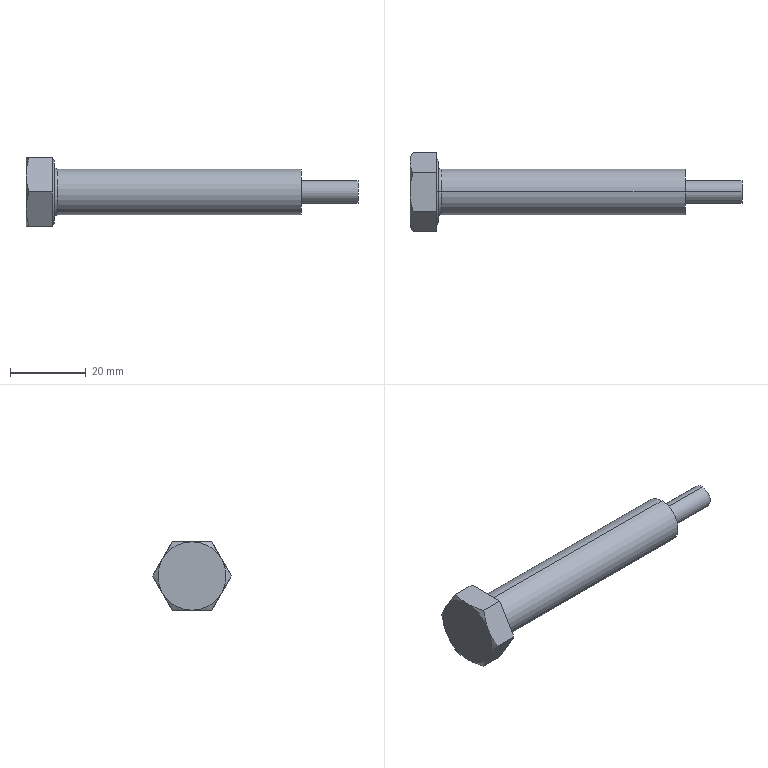Part | SolidWorks | features Chamfer 2, ICE 2, RevCut 2, Revolution 2, Extrusion 1 | 1 solid | 25 faces | box 87.5 x 20.785 x 18 mm | volume 9848 mm3 | plane 11 | cone 8 | cylinder 4 | torus 2 | commonest cylinder face diameters 6 x2 12 x2
STEP:
#1=CARTESIAN_POINT('',(72.5,0.,-3.));
#2=VERTEX_POINT('',#1);
#3=CARTESIAN_POINT('',(72.5,0.,3.));
#4=VERTEX_POINT('',#3);
#5=CARTESIAN_POINT('',(72.5,0.,0.));
#6=DIRECTION('',(1.,0.,0.));
#7=DIRECTION('',(0.,0.,-1.));
#8=AXIS2_PLACEMENT_3D('',#5,#6,#7);
#9=CIRCLE('',#8,3.);
#10=EDGE_CURVE('',#2,#4,#9,.T.);
#11=ORIENTED_EDGE('',*,*,#10,.T.);
#12=CARTESIAN_POINT('',(87.5,0.,3.));
#13=VERTEX_POINT('',#12);
#14=CARTESIAN_POINT('',(72.5,0.,3.));
#15=DIRECTION('',(1.,0.,0.));
#16=VECTOR('',#15,1000.);
#17=LINE('',#14,#16);
#18=EDGE_CURVE('',#4,#13,#17,.T.);
#19=ORIENTED_EDGE('',*,*,#18,.T.);
#20=CARTESIAN_POINT('',(87.5,0.,-3.));
#21=VERTEX_POINT('',#20);
#22=CARTESIAN_POINT('',(87.5,0.,0.));
#23=DIRECTION('',(1.,0.,0.));
#24=DIRECTION('',(0.,0.,-1.));
#25=AXIS2_PLACEMENT_3D('',#22,#23,#24);
#26=CIRCLE('',#25,3.);
#27=EDGE_CURVE('',#21,#13,#26,.T.);
#28=ORIENTED_EDGE('',*,*,#27,.F.);
#29=CARTESIAN_POINT('',(72.5,0.,-3.));
#30=DIRECTION('',(1.,0.,0.));
#31=VECTOR('',#30,1000.);
#32=LINE('',#29,#31);
#33=EDGE_CURVE('',#2,#21,#32,.T.);
#34=ORIENTED_EDGE('',*,*,#33,.F.);
#35=EDGE_LOOP('',(#11,#19,#28,#34));
#36=FACE_OUTER_BOUND('',#35,.T.);
#37=CARTESIAN_POINT('',(72.5,0.,0.));
#38=DIRECTION('',(1.,0.,0.));
#39=DIRECTION('',(0.,0.,-1.));
#40=AXIS2_PLACEMENT_3D('',#37,#38,#39);
#41=CYLINDRICAL_SURFACE('',#40,3.);
#42=ADVANCED_FACE('',(#36),#41,.T.);
#43=CARTESIAN_POINT('',(7.5,0.,8.215));
#44=VERTEX_POINT('',#43);
#45=CARTESIAN_POINT('',(7.5,0.,-8.215));
#46=VERTEX_POINT('',#45);
#47=CARTESIAN_POINT('',(7.5,0.,0.));
#48=DIRECTION('',(-1.,0.,0.));
#49=DIRECTION('',(0.,0.,1.));
#50=AXIS2_PLACEMENT_3D('',#47,#48,#49);
#51=CIRCLE('',#50,8.215);
#52=EDGE_CURVE('',#44,#46,#51,.T.);
#53=ORIENTED_EDGE('',*,*,#52,.T.);
#54=CARTESIAN_POINT('',(6.9,0.,-8.815));
#55=VERTEX_POINT('',#54);
#56=CARTESIAN_POINT('',(6.9,0.,-8.815));
#57=DIRECTION('',(-0.7071,0.,-0.7071));
#58=VECTOR('',#57,1000.);
#59=LINE('',#56,#58);
#60=EDGE_CURVE('',#46,#55,#59,.T.);
#61=ORIENTED_EDGE('',*,*,#60,.T.);
#62=CARTESIAN_POINT('',(6.9,0.,8.815));
#63=VERTEX_POINT('',#62);
#64=CARTESIAN_POINT('',(6.9,0.,0.));
#65=DIRECTION('',(-1.,0.,0.));
#66=DIRECTION('',(0.,0.,1.));
#67=AXIS2_PLACEMENT_3D('',#64,#65,#66);
#68=CIRCLE('',#67,8.815);
#69=EDGE_CURVE('',#63,#55,#68,.T.);
#70=ORIENTED_EDGE('',*,*,#69,.F.);
#71=CARTESIAN_POINT('',(6.9,0.,8.815));
#72=DIRECTION('',(-0.7071,0.,0.7071));
#73=VECTOR('',#72,1000.);
#74=LINE('',#71,#73);
#75=EDGE_CURVE('',#44,#63,#74,.T.);
#76=ORIENTED_EDGE('',*,*,#75,.F.);
#77=EDGE_LOOP('',(#53,#61,#70,#76));
#78=FACE_OUTER_BOUND('',#77,.T.);
#79=CARTESIAN_POINT('',(6.9,0.,0.));
#80=DIRECTION('',(-1.,0.,0.));
#81=DIRECTION('',(0.,0.,1.));
#82=AXIS2_PLACEMENT_3D('',#79,#80,#81);
#83=CONICAL_SURFACE('',#82,8.815,0.7854);
#84=ADVANCED_FACE('',(#78),#83,.T.);
#85=CARTESIAN_POINT('',(7.5,0.,-6.85));
#86=VERTEX_POINT('',#85);
#87=CARTESIAN_POINT('',(7.5,0.,6.85));
#88=VERTEX_POINT('',#87);
#89=CARTESIAN_POINT('',(7.5,0.,0.));
#90=DIRECTION('',(-1.,0.,0.));
#91=DIRECTION('',(0.,0.,1.));
#92=AXIS2_PLACEMENT_3D('',#89,#90,#91);
#93=CIRCLE('',#92,6.85);
#94=EDGE_CURVE('',#86,#88,#93,.T.);
#95=ORIENTED_EDGE('',*,*,#94,.F.);
#96=CARTESIAN_POINT('',(8.35,0.,-6.));
#97=VERTEX_POINT('',#96);
#98=CARTESIAN_POINT('',(8.35,0.,-6.85));
#99=DIRECTION('',(0.,1.,0.));
#100=DIRECTION('',(0.,0.,1.));
#101=AXIS2_PLACEMENT_3D('',#98,#99,#100);
#102=CIRCLE('',#101,0.85);
#103=EDGE_CURVE('',#86,#97,#102,.T.);
#104=ORIENTED_EDGE('',*,*,#103,.T.);
#105=CARTESIAN_POINT('',(8.35,0.,6.));
#106=VERTEX_POINT('',#105);
#107=CARTESIAN_POINT('',(8.35,0.,0.));
#108=DIRECTION('',(-1.,0.,0.));
#109=DIRECTION('',(0.,0.,1.));
#110=AXIS2_PLACEMENT_3D('',#107,#108,#109);
#111=CIRCLE('',#110,6.);
#112=EDGE_CURVE('',#97,#106,#111,.T.);
#113=ORIENTED_EDGE('',*,*,#112,.T.);
#114=CARTESIAN_POINT('',(8.35,0.,6.85));
#115=DIRECTION('',(0.,-1.,0.));
#116=DIRECTION('',(0.,0.,-1.));
#117=AXIS2_PLACEMENT_3D('',#114,#115,#116);
#118=CIRCLE('',#117,0.85);
#119=EDGE_CURVE('',#88,#106,#118,.T.);
#120=ORIENTED_EDGE('',*,*,#119,.F.);
#121=EDGE_LOOP('',(#95,#104,#113,#120));
#122=FACE_OUTER_BOUND('',#121,.T.);
#123=CARTESIAN_POINT('',(8.35,0.,0.));
#124=DIRECTION('',(-1.,0.,0.));
#125=DIRECTION('',(0.,0.,1.));
#126=AXIS2_PLACEMENT_3D('',#123,#124,#125);
#127=TOROIDAL_SURFACE('',#126,6.85,0.85);
#128=ADVANCED_FACE('',(#122),#127,.F.);
#129=CARTESIAN_POINT('',(72.5,0.,-6.));
#130=VERTEX_POINT('',#129);
#131=CARTESIAN_POINT('',(72.5,0.,6.));
#132=VERTEX_POINT('',#131);
#133=CARTESIAN_POINT('',(72.5,0.,0.));
#134=DIRECTION('',(1.,0.,0.));
#135=DIRECTION('',(0.,0.,-1.));
#136=AXIS2_PLACEMENT_3D('',#133,#134,#135);
#137=CIRCLE('',#136,6.);
#138=EDGE_CURVE('',#130,#132,#137,.T.);
#139=ORIENTED_EDGE('',*,*,#138,.F.);
#140=CARTESIAN_POINT('',(7.5,0.,-6.));
#141=DIRECTION('',(-1.,0.,0.));
#142=VECTOR('',#141,1000.);
#143=LINE('',#140,#142);
#144=EDGE_CURVE('',#130,#97,#143,.T.);
#145=ORIENTED_EDGE('',*,*,#144,.T.);
#146=CARTESIAN_POINT('',(8.35,0.,0.));
#147=DIRECTION('',(-1.,0.,0.));
#148=DIRECTION('',(0.,0.,1.));
#149=AXIS2_PLACEMENT_3D('',#146,#147,#148);
#150=CIRCLE('',#149,6.);
#151=EDGE_CURVE('',#106,#97,#150,.T.);
#152=ORIENTED_EDGE('',*,*,#151,.F.);
#153=CARTESIAN_POINT('',(7.5,0.,6.));
#154=DIRECTION('',(-1.,0.,0.));
#155=VECTOR('',#154,1000.);
#156=LINE('',#153,#155);
#157=EDGE_CURVE('',#132,#106,#156,.T.);
#158=ORIENTED_EDGE('',*,*,#157,.F.);
#159=EDGE_LOOP('',(#139,#145,#152,#158));
#160=FACE_OUTER_BOUND('',#159,.T.);
#161=CARTESIAN_POINT('',(7.5,0.,0.));
#162=DIRECTION('',(-1.,0.,0.));
#163=DIRECTION('',(0.,0.,1.));
#164=AXIS2_PLACEMENT_3D('',#161,#162,#163);
#165=CYLINDRICAL_SURFACE('',#164,6.);
#166=ADVANCED_FACE('',(#160),#165,.T.);
#167=ORIENTED_EDGE('',*,*,#144,.F.);
#168=CARTESIAN_POINT('',(72.5,0.,0.));
#169=DIRECTION('',(1.,0.,0.));
#170=DIRECTION('',(0.,0.,-1.));
#171=AXIS2_PLACEMENT_3D('',#168,#169,#170);
#172=CIRCLE('',#171,6.);
#173=EDGE_CURVE('',#132,#130,#172,.T.);
#174=ORIENTED_EDGE('',*,*,#173,.F.);
#175=ORIENTED_EDGE('',*,*,#157,.T.);
#176=ORIENTED_EDGE('',*,*,#112,.F.);
#177=EDGE_LOOP('',(#167,#174,#175,#176));
#178=FACE_OUTER_BOUND('',#177,.T.);
#179=CARTESIAN_POINT('',(7.5,0.,0.));
#180=DIRECTION('',(-1.,0.,0.));
#181=DIRECTION('',(0.,0.,1.));
#182=AXIS2_PLACEMENT_3D('',#179,#180,#181);
#183=CYLINDRICAL_SURFACE('',#182,6.);
#184=ADVANCED_FACE('',(#178),#183,.T.);
#185=CARTESIAN_POINT('',(7.5,0.,0.));
#186=DIRECTION('',(-1.,0.,0.));
#187=DIRECTION('',(0.,0.,1.));
#188=AXIS2_PLACEMENT_3D('',#185,#186,#187);
#189=CIRCLE('',#188,6.85);
#190=EDGE_CURVE('',#88,#86,#189,.T.);
#191=ORIENTED_EDGE('',*,*,#190,.T.);
#192=ORIENTED_EDGE('',*,*,#94,.T.);
#193=EDGE_LOOP('',(#191,#192));
#194=FACE_BOUND('',#193,.T.);
#195=ORIENTED_EDGE('',*,*,#52,.F.);
#196=CARTESIAN_POINT('',(7.5,0.,0.));
#197=DIRECTION('',(-1.,0.,0.));
#198=DIRECTION('',(0.,0.,1.));
#199=AXIS2_PLACEMENT_3D('',#196,#197,#198);
#200=CIRCLE('',#199,8.215);
#201=EDGE_CURVE('',#46,#44,#200,.T.);
#202=ORIENTED_EDGE('',*,*,#201,.F.);
#203=EDGE_LOOP('',(#195,#202));
#204=FACE_OUTER_BOUND('',#203,.T.);
#205=CARTESIAN_POINT('',(7.5,5.196,-9.));
#206=DIRECTION('',(1.,0.,0.));
#207=DIRECTION('',(0.,0.,-1.));
#208=AXIS2_PLACEMENT_3D('',#205,#206,#207);
#209=PLANE('',#208);
#210=ADVANCED_FACE('',(#194,#204),#209,.T.);
#211=ORIENTED_EDGE('',*,*,#103,.F.);
#212=ORIENTED_EDGE('',*,*,#190,.F.);
#213=ORIENTED_EDGE('',*,*,#119,.T.);
#214=ORIENTED_EDGE('',*,*,#151,.T.);
#215=EDGE_LOOP('',(#211,#212,#213,#214));
#216=FACE_OUTER_BOUND('',#215,.T.);
#217=CARTESIAN_POINT('',(8.35,0.,0.));
#218=DIRECTION('',(-1.,0.,0.));
#219=DIRECTION('',(0.,0.,1.));
#220=AXIS2_PLACEMENT_3D('',#217,#218,#219);
#221=TOROIDAL_SURFACE('',#220,6.85,0.85);
#222=ADVANCED_FACE('',(#216),#221,.F.);
#223=ORIENTED_EDGE('',*,*,#69,.T.);
#224=CARTESIAN_POINT('',(6.9,0.,0.));
#225=DIRECTION('',(-1.,0.,0.));
#226=DIRECTION('',(0.,0.,1.));
#227=AXIS2_PLACEMENT_3D('',#224,#225,#226);
#228=CIRCLE('',#227,8.815);
#229=EDGE_CURVE('',#55,#63,#228,.T.);
#230=ORIENTED_EDGE('',*,*,#229,.T.);
#231=EDGE_LOOP('',(#223,#230));
#232=FACE_BOUND('',#231,.T.);
#233=CARTESIAN_POINT('',(6.9,-5.196,-9.));
#234=VERTEX_POINT('',#233);
#235=CARTESIAN_POINT('',(6.9,5.196,-9.));
#236=VERTEX_POINT('',#235);
#237=CARTESIAN_POINT('',(6.9,-5.196,-9.));
#238=DIRECTION('',(0.,1.,0.));
#239=VECTOR('',#238,1000.);
#240=LINE('',#237,#239);
#241=EDGE_CURVE('',#234,#236,#240,.T.);
#242=ORIENTED_EDGE('',*,*,#241,.T.);
#243=CARTESIAN_POINT('',(6.9,10.392,0.));
#244=VERTEX_POINT('',#243);
#245=CARTESIAN_POINT('',(6.9,5.196,-9.));
#246=DIRECTION('',(0.,0.5,0.866));
#247=VECTOR('',#246,1000.);
#248=LINE('',#245,#247);
#249=EDGE_CURVE('',#236,#244,#248,.T.);
#250=ORIENTED_EDGE('',*,*,#249,.T.);
#251=CARTESIAN_POINT('',(6.9,5.196,9.));
#252=VERTEX_POINT('',#251);
#253=CARTESIAN_POINT('',(6.9,10.392,0.));
#254=DIRECTION('',(0.,-0.5,0.866));
#255=VECTOR('',#254,1000.);
#256=LINE('',#253,#255);
#257=EDGE_CURVE('',#244,#252,#256,.T.);
#258=ORIENTED_EDGE('',*,*,#257,.T.);
#259=CARTESIAN_POINT('',(6.9,-5.196,9.));
#260=VERTEX_POINT('',#259);
#261=CARTESIAN_POINT('',(6.9,5.196,9.));
#262=DIRECTION('',(0.,-1.,0.));
#263=VECTOR('',#262,1000.);
#264=LINE('',#261,#263);
#265=EDGE_CURVE('',#252,#260,#264,.T.);
#266=ORIENTED_EDGE('',*,*,#265,.T.);
#267=CARTESIAN_POINT('',(6.9,-10.392,0.));
#268=VERTEX_POINT('',#267);
#269=CARTESIAN_POINT('',(6.9,-5.196,9.));
#270=DIRECTION('',(0.,-0.5,-0.866));
#271=VECTOR('',#270,1000.);
#272=LINE('',#269,#271);
#273=EDGE_CURVE('',#260,#268,#272,.T.);
#274=ORIENTED_EDGE('',*,*,#273,.T.);
#275=CARTESIAN_POINT('',(6.9,-10.392,0.));
#276=DIRECTION('',(0.,0.5,-0.866));
#277=VECTOR('',#276,1000.);
#278=LINE('',#275,#277);
#279=EDGE_CURVE('',#268,#234,#278,.T.);
#280=ORIENTED_EDGE('',*,*,#279,.T.);
#281=EDGE_LOOP('',(#242,#250,#258,#266,#274,#280));
#282=FACE_OUTER_BOUND('',#281,.T.);
#283=CARTESIAN_POINT('',(6.9,-8.815,0.));
#284=DIRECTION('',(1.,0.,0.));
#285=DIRECTION('',(0.,0.,-1.));
#286=AXIS2_PLACEMENT_3D('',#283,#284,#285);
#287=PLANE('',#286);
#288=ADVANCED_FACE('',(#232,#282),#287,.T.);
#289=ORIENTED_EDGE('',*,*,#60,.F.);
#290=ORIENTED_EDGE('',*,*,#201,.T.);
#291=ORIENTED_EDGE('',*,*,#75,.T.);
#292=ORIENTED_EDGE('',*,*,#229,.F.);
#293=EDGE_LOOP('',(#289,#290,#291,#292));
#294=FACE_OUTER_BOUND('',#293,.T.);
#295=CARTESIAN_POINT('',(6.9,0.,0.));
#296=DIRECTION('',(-1.,0.,0.));
#297=DIRECTION('',(0.,0.,1.));
#298=AXIS2_PLACEMENT_3D('',#295,#296,#297);
#299=CONICAL_SURFACE('',#298,8.815,0.7854);
#300=ADVANCED_FACE('',(#294),#299,.T.);
#301=CARTESIAN_POINT('',(0.,0.,-9.));
#302=VERTEX_POINT('',#301);
#303=CARTESIAN_POINT('',(0.,7.794,-4.5));
#304=VERTEX_POINT('',#303);
#305=CARTESIAN_POINT('',(0.,0.,0.));
#306=DIRECTION('',(1.,0.,0.));
#307=DIRECTION('',(0.,0.,-1.));
#308=AXIS2_PLACEMENT_3D('',#305,#306,#307);
#309=CIRCLE('',#308,9.);
#310=EDGE_CURVE('',#302,#304,#309,.T.);
#311=ORIENTED_EDGE('',*,*,#310,.F.);
#312=CARTESIAN_POINT('',(0.,-7.794,-4.5));
#313=VERTEX_POINT('',#312);
#314=CARTESIAN_POINT('',(0.,0.,0.));
#315=DIRECTION('',(1.,0.,0.));
#316=DIRECTION('',(0.,0.,-1.));
#317=AXIS2_PLACEMENT_3D('',#314,#315,#316);
#318=CIRCLE('',#317,9.);
#319=EDGE_CURVE('',#313,#302,#318,.T.);
#320=ORIENTED_EDGE('',*,*,#319,.F.);
#321=CARTESIAN_POINT('',(0.,-7.794,4.5));
#322=VERTEX_POINT('',#321);
#323=CARTESIAN_POINT('',(0.,0.,0.));
#324=DIRECTION('',(1.,0.,0.));
#325=DIRECTION('',(0.,0.,-1.));
#326=AXIS2_PLACEMENT_3D('',#323,#324,#325);
#327=CIRCLE('',#326,9.);
#328=EDGE_CURVE('',#322,#313,#327,.T.);
#329=ORIENTED_EDGE('',*,*,#328,.F.);
#330=CARTESIAN_POINT('',(0.,0.,9.));
#331=VERTEX_POINT('',#330);
#332=CARTESIAN_POINT('',(0.,0.,0.));
#333=DIRECTION('',(1.,0.,0.));
#334=DIRECTION('',(0.,0.,-1.));
#335=AXIS2_PLACEMENT_3D('',#332,#333,#334);
#336=CIRCLE('',#335,9.);
#337=EDGE_CURVE('',#331,#322,#336,.T.);
#338=ORIENTED_EDGE('',*,*,#337,.F.);
#339=CARTESIAN_POINT('',(0.,7.794,4.5));
#340=VERTEX_POINT('',#339);
#341=CARTESIAN_POINT('',(0.,0.,0.));
#342=DIRECTION('',(-1.,0.,0.));
#343=DIRECTION('',(0.,0.,1.));
#344=AXIS2_PLACEMENT_3D('',#341,#342,#343);
#345=CIRCLE('',#344,9.);
#346=EDGE_CURVE('',#331,#340,#345,.T.);
#347=ORIENTED_EDGE('',*,*,#346,.T.);
#348=CARTESIAN_POINT('',(0.,0.,0.));
#349=DIRECTION('',(1.,0.,0.));
#350=DIRECTION('',(0.,0.,-1.));
#351=AXIS2_PLACEMENT_3D('',#348,#349,#350);
#352=CIRCLE('',#351,9.);
#353=EDGE_CURVE('',#304,#340,#352,.T.);
#354=ORIENTED_EDGE('',*,*,#353,.F.);
#355=EDGE_LOOP('',(#311,#320,#329,#338,#347,#354));
#356=FACE_OUTER_BOUND('',#355,.T.);
#357=CARTESIAN_POINT('',(0.,5.196,-9.));
#358=DIRECTION('',(1.,0.,0.));
#359=DIRECTION('',(0.,0.,-1.));
#360=AXIS2_PLACEMENT_3D('',#357,#358,#359);
#361=PLANE('',#360);
#362=ADVANCED_FACE('',(#356),#361,.F.);
#363=CARTESIAN_POINT('',(0.8038,5.196,-9.));
#364=VERTEX_POINT('',#363);
#365=CARTESIAN_POINT('',(0.,7.794,-4.5));
#366=CARTESIAN_POINT('',(0.,7.574,-4.882));
#367=CARTESIAN_POINT('',(0.019,7.352,-5.266));
#368=CARTESIAN_POINT('',(0.09253,6.914,-6.024));
#369=CARTESIAN_POINT('',(0.147,6.697,-6.401));
#370=CARTESIAN_POINT('',(0.357,6.048,-7.525));
#371=CARTESIAN_POINT('',(0.5591,5.62,-8.266));
#372=CARTESIAN_POINT('',(0.8038,5.196,-9.));
#373=B_SPLINE_CURVE_WITH_KNOTS('',3,(#365,#366,#367,#368,#369,#370,#371,#372),.UNSPECIFIED.,.F.,.F.,(4,2,2,4),(0.005258,0.006567,0.007877,0.0105),.UNSPECIFIED.);
#374=EDGE_CURVE('',#304,#364,#373,.T.);
#375=ORIENTED_EDGE('',*,*,#374,.T.);
#376=CARTESIAN_POINT('',(0.8038,5.196,-9.));
#377=CARTESIAN_POINT('',(0.5613,4.356,-9.));
#378=CARTESIAN_POINT('',(0.3593,3.505,-9.));
#379=CARTESIAN_POINT('',(0.07758,1.769,-9.));
#380=CARTESIAN_POINT('',(0.,0.8787,-9.));
#381=CARTESIAN_POINT('',(0.,0.,-9.));
#382=B_SPLINE_CURVE_WITH_KNOTS('',3,(#376,#377,#378,#379,#380,#381),.UNSPECIFIED.,.F.,.F.,(4,2,4),(0.003787,0.00641,0.009033),.UNSPECIFIED.);
#383=EDGE_CURVE('',#364,#302,#382,.T.);
#384=ORIENTED_EDGE('',*,*,#383,.T.);
#385=ORIENTED_EDGE('',*,*,#310,.T.);
#386=EDGE_LOOP('',(#375,#384,#385));
#387=FACE_OUTER_BOUND('',#386,.T.);
#388=CARTESIAN_POINT('',(0.,0.,0.));
#389=DIRECTION('',(1.,0.,0.));
#390=DIRECTION('',(0.,0.,1.));
#391=AXIS2_PLACEMENT_3D('',#388,#389,#390);
#392=CONICAL_SURFACE('',#391,9.,1.047);
#393=ADVANCED_FACE('',(#387),#392,.T.);
#394=CARTESIAN_POINT('',(0.8038,10.392,0.));
#395=VERTEX_POINT('',#394);
#396=CARTESIAN_POINT('',(0.,7.794,4.5));
#397=CARTESIAN_POINT('',(0.,8.015,4.118));
#398=CARTESIAN_POINT('',(0.019,8.236,3.734));
#399=CARTESIAN_POINT('',(0.09253,8.674,2.976));
#400=CARTESIAN_POINT('',(0.147,8.892,2.599));
#401=CARTESIAN_POINT('',(0.357,9.541,1.475));
#402=CARTESIAN_POINT('',(0.5591,9.968,0.7343));
#403=CARTESIAN_POINT('',(0.8038,10.392,0.));
#404=B_SPLINE_CURVE_WITH_KNOTS('',3,(#396,#397,#398,#399,#400,#401,#402,#403),.UNSPECIFIED.,.F.,.F.,(4,2,2,4),(0.005258,0.006567,0.007877,0.0105),.UNSPECIFIED.);
#405=EDGE_CURVE('',#340,#395,#404,.T.);
#406=ORIENTED_EDGE('',*,*,#405,.T.);
#407=CARTESIAN_POINT('',(0.8038,10.392,0.));
#408=CARTESIAN_POINT('',(0.5585,9.967,-0.7361));
#409=CARTESIAN_POINT('',(0.3563,9.539,-1.478));
#410=CARTESIAN_POINT('',(0.07661,8.674,-2.976));
#411=CARTESIAN_POINT('',(0.,8.237,-3.733));
#412=CARTESIAN_POINT('',(0.,7.794,-4.5));
#413=B_SPLINE_CURVE_WITH_KNOTS('',3,(#407,#408,#409,#410,#411,#412),.UNSPECIFIED.,.F.,.F.,(4,2,4),(0.000000238,0.002629,0.005258),.UNSPECIFIED.);
#414=EDGE_CURVE('',#395,#304,#413,.T.);
#415=ORIENTED_EDGE('',*,*,#414,.T.);
#416=ORIENTED_EDGE('',*,*,#353,.T.);
#417=EDGE_LOOP('',(#406,#415,#416));
#418=FACE_OUTER_BOUND('',#417,.T.);
#419=CARTESIAN_POINT('',(0.,0.,0.));
#420=DIRECTION('',(1.,0.,0.));
#421=DIRECTION('',(0.,0.,1.));
#422=AXIS2_PLACEMENT_3D('',#419,#420,#421);
#423=CONICAL_SURFACE('',#422,9.,1.047);
#424=ADVANCED_FACE('',(#418),#423,.T.);
#425=CARTESIAN_POINT('',(0.8038,5.196,9.));
#426=VERTEX_POINT('',#425);
#427=CARTESIAN_POINT('',(0.8038,5.196,9.));
#428=CARTESIAN_POINT('',(0.5585,5.621,8.264));
#429=CARTESIAN_POINT('',(0.3563,6.049,7.522));
#430=CARTESIAN_POINT('',(0.07661,6.914,6.024));
#431=CARTESIAN_POINT('',(0.,7.352,5.267));
#432=CARTESIAN_POINT('',(0.,7.794,4.5));
#433=B_SPLINE_CURVE_WITH_KNOTS('',3,(#427,#428,#429,#430,#431,#432),.UNSPECIFIED.,.F.,.F.,(4,2,4),(0.000000238,0.002629,0.005258),.UNSPECIFIED.);
#434=EDGE_CURVE('',#426,#340,#433,.T.);
#435=ORIENTED_EDGE('',*,*,#434,.T.);
#436=ORIENTED_EDGE('',*,*,#346,.F.);
#437=CARTESIAN_POINT('',(0.,0.,9.));
#438=CARTESIAN_POINT('',(0.,0.8787,9.));
#439=CARTESIAN_POINT('',(0.07758,1.769,9.));
#440=CARTESIAN_POINT('',(0.3593,3.505,9.));
#441=CARTESIAN_POINT('',(0.5613,4.356,9.));
#442=CARTESIAN_POINT('',(0.8038,5.196,9.));
#443=B_SPLINE_CURVE_WITH_KNOTS('',3,(#437,#438,#439,#440,#441,#442),.UNSPECIFIED.,.F.,.F.,(4,2,4),(0.01455,0.01718,0.01981),.UNSPECIFIED.);
#444=EDGE_CURVE('',#331,#426,#443,.T.);
#445=ORIENTED_EDGE('',*,*,#444,.T.);
#446=EDGE_LOOP('',(#435,#436,#445));
#447=FACE_OUTER_BOUND('',#446,.T.);
#448=CARTESIAN_POINT('',(0.,0.,0.));
#449=DIRECTION('',(1.,0.,0.));
#450=DIRECTION('',(0.,0.,1.));
#451=AXIS2_PLACEMENT_3D('',#448,#449,#450);
#452=CONICAL_SURFACE('',#451,9.,1.047);
#453=ADVANCED_FACE('',(#447),#452,.T.);
#454=CARTESIAN_POINT('',(0.8038,-5.196,9.));
#455=VERTEX_POINT('',#454);
#456=CARTESIAN_POINT('',(0.8038,-5.196,9.));
#457=CARTESIAN_POINT('',(0.5599,-4.351,9.));
#458=CARTESIAN_POINT('',(0.3553,-3.485,9.));
#459=CARTESIAN_POINT('',(0.07548,-1.75,9.));
#460=CARTESIAN_POINT('',(0.,-0.8781,9.));
#461=CARTESIAN_POINT('',(0.,0.,9.));
#462=B_SPLINE_CURVE_WITH_KNOTS('',3,(#456,#457,#458,#459,#460,#461),.UNSPECIFIED.,.F.,.F.,(4,2,4),(0.009291,0.01192,0.01455),.UNSPECIFIED.);
#463=EDGE_CURVE('',#455,#331,#462,.T.);
#464=ORIENTED_EDGE('',*,*,#463,.T.);
#465=ORIENTED_EDGE('',*,*,#337,.T.);
#466=CARTESIAN_POINT('',(0.,-7.794,4.5));
#467=CARTESIAN_POINT('',(0.,-7.574,4.882));
#468=CARTESIAN_POINT('',(0.019,-7.352,5.266));
#469=CARTESIAN_POINT('',(0.09253,-6.914,6.024));
#470=CARTESIAN_POINT('',(0.147,-6.697,6.401));
#471=CARTESIAN_POINT('',(0.357,-6.048,7.525));
#472=CARTESIAN_POINT('',(0.5591,-5.62,8.266));
#473=CARTESIAN_POINT('',(0.8038,-5.196,9.));
#474=B_SPLINE_CURVE_WITH_KNOTS('',3,(#466,#467,#468,#469,#470,#471,#472,#473),.UNSPECIFIED.,.F.,.F.,(4,2,2,4),(0.005258,0.006567,0.007877,0.0105),.UNSPECIFIED.);
#475=EDGE_CURVE('',#322,#455,#474,.T.);
#476=ORIENTED_EDGE('',*,*,#475,.T.);
#477=EDGE_LOOP('',(#464,#465,#476));
#478=FACE_OUTER_BOUND('',#477,.T.);
#479=CARTESIAN_POINT('',(0.,0.,0.));
#480=DIRECTION('',(1.,0.,0.));
#481=DIRECTION('',(0.,0.,1.));
#482=AXIS2_PLACEMENT_3D('',#479,#480,#481);
#483=CONICAL_SURFACE('',#482,9.,1.047);
#484=ADVANCED_FACE('',(#478),#483,.T.);
#485=CARTESIAN_POINT('',(0.8038,-5.196,-9.));
#486=VERTEX_POINT('',#485);
#487=CARTESIAN_POINT('',(0.,0.,-9.));
#488=CARTESIAN_POINT('',(0.,-0.8781,-9.));
#489=CARTESIAN_POINT('',(0.07548,-1.75,-9.));
#490=CARTESIAN_POINT('',(0.3553,-3.485,-9.));
#491=CARTESIAN_POINT('',(0.5599,-4.351,-9.));
#492=CARTESIAN_POINT('',(0.8038,-5.196,-9.));
#493=B_SPLINE_CURVE_WITH_KNOTS('',3,(#487,#488,#489,#490,#491,#492),.UNSPECIFIED.,.F.,.F.,(4,2,4),(0.009033,0.01165,0.01428),.UNSPECIFIED.);
#494=EDGE_CURVE('',#302,#486,#493,.T.);
#495=ORIENTED_EDGE('',*,*,#494,.T.);
#496=CARTESIAN_POINT('',(0.8038,-5.196,-9.));
#497=CARTESIAN_POINT('',(0.5585,-5.621,-8.264));
#498=CARTESIAN_POINT('',(0.3563,-6.049,-7.522));
#499=CARTESIAN_POINT('',(0.07661,-6.914,-6.024));
#500=CARTESIAN_POINT('',(0.,-7.352,-5.267));
#501=CARTESIAN_POINT('',(0.,-7.794,-4.5));
#502=B_SPLINE_CURVE_WITH_KNOTS('',3,(#496,#497,#498,#499,#500,#501),.UNSPECIFIED.,.F.,.F.,(4,2,4),(0.000000238,0.002629,0.005258),.UNSPECIFIED.);
#503=EDGE_CURVE('',#486,#313,#502,.T.);
#504=ORIENTED_EDGE('',*,*,#503,.T.);
#505=ORIENTED_EDGE('',*,*,#319,.T.);
#506=EDGE_LOOP('',(#495,#504,#505));
#507=FACE_OUTER_BOUND('',#506,.T.);
#508=CARTESIAN_POINT('',(0.,0.,0.));
#509=DIRECTION('',(1.,0.,0.));
#510=DIRECTION('',(0.,0.,1.));
#511=AXIS2_PLACEMENT_3D('',#508,#509,#510);
#512=CONICAL_SURFACE('',#511,9.,1.047);
#513=ADVANCED_FACE('',(#507),#512,.T.);
#514=CARTESIAN_POINT('',(0.8038,-10.392,0.));
#515=VERTEX_POINT('',#514);
#516=CARTESIAN_POINT('',(0.8038,-10.392,0.));
#517=CARTESIAN_POINT('',(0.5585,-9.967,0.7361));
#518=CARTESIAN_POINT('',(0.3563,-9.539,1.478));
#519=CARTESIAN_POINT('',(0.07661,-8.674,2.976));
#520=CARTESIAN_POINT('',(0.,-8.237,3.733));
#521=CARTESIAN_POINT('',(0.,-7.794,4.5));
#522=B_SPLINE_CURVE_WITH_KNOTS('',3,(#516,#517,#518,#519,#520,#521),.UNSPECIFIED.,.F.,.F.,(4,2,4),(0.000000238,0.002629,0.005258),.UNSPECIFIED.);
#523=EDGE_CURVE('',#515,#322,#522,.T.);
#524=ORIENTED_EDGE('',*,*,#523,.T.);
#525=ORIENTED_EDGE('',*,*,#328,.T.);
#526=CARTESIAN_POINT('',(0.,-7.794,-4.5));
#527=CARTESIAN_POINT('',(0.,-8.015,-4.118));
#528=CARTESIAN_POINT('',(0.019,-8.236,-3.734));
#529=CARTESIAN_POINT('',(0.09253,-8.674,-2.976));
#530=CARTESIAN_POINT('',(0.147,-8.892,-2.599));
#531=CARTESIAN_POINT('',(0.357,-9.541,-1.475));
#532=CARTESIAN_POINT('',(0.5591,-9.968,-0.7343));
#533=CARTESIAN_POINT('',(0.8038,-10.392,0.));
#534=B_SPLINE_CURVE_WITH_KNOTS('',3,(#526,#527,#528,#529,#530,#531,#532,#533),.UNSPECIFIED.,.F.,.F.,(4,2,2,4),(0.005258,0.006567,0.007877,0.0105),.UNSPECIFIED.);
#535=EDGE_CURVE('',#313,#515,#534,.T.);
#536=ORIENTED_EDGE('',*,*,#535,.T.);
#537=EDGE_LOOP('',(#524,#525,#536));
#538=FACE_OUTER_BOUND('',#537,.T.);
#539=CARTESIAN_POINT('',(0.,0.,0.));
#540=DIRECTION('',(1.,0.,0.));
#541=DIRECTION('',(0.,0.,1.));
#542=AXIS2_PLACEMENT_3D('',#539,#540,#541);
#543=CONICAL_SURFACE('',#542,9.,1.047);
#544=ADVANCED_FACE('',(#538),#543,.T.);
#545=ORIENTED_EDGE('',*,*,#279,.F.);
#546=CARTESIAN_POINT('',(7.5,-10.392,0.));
#547=DIRECTION('',(-1.,0.,0.));
#548=VECTOR('',#547,1000.);
#549=LINE('',#546,#548);
#550=EDGE_CURVE('',#268,#515,#549,.T.);
#551=ORIENTED_EDGE('',*,*,#550,.T.);
#552=ORIENTED_EDGE('',*,*,#535,.F.);
#553=ORIENTED_EDGE('',*,*,#503,.F.);
#554=CARTESIAN_POINT('',(7.5,-5.196,-9.));
#555=DIRECTION('',(-1.,0.,0.));
#556=VECTOR('',#555,1000.);
#557=LINE('',#554,#556);
#558=EDGE_CURVE('',#234,#486,#557,.T.);
#559=ORIENTED_EDGE('',*,*,#558,.F.);
#560=EDGE_LOOP('',(#545,#551,#552,#553,#559));
#561=FACE_OUTER_BOUND('',#560,.T.);
#562=CARTESIAN_POINT('',(7.5,-10.392,0.));
#563=DIRECTION('',(0.,0.866,0.5));
#564=DIRECTION('',(0.,-0.5,0.866));
#565=AXIS2_PLACEMENT_3D('',#562,#563,#564);
#566=PLANE('',#565);
#567=ADVANCED_FACE('',(#561),#566,.F.);
#568=ORIENTED_EDGE('',*,*,#273,.F.);
#569=CARTESIAN_POINT('',(7.5,-5.196,9.));
#570=DIRECTION('',(-1.,0.,0.));
#571=VECTOR('',#570,1000.);
#572=LINE('',#569,#571);
#573=EDGE_CURVE('',#260,#455,#572,.T.);
#574=ORIENTED_EDGE('',*,*,#573,.T.);
#575=ORIENTED_EDGE('',*,*,#475,.F.);
#576=ORIENTED_EDGE('',*,*,#523,.F.);
#577=ORIENTED_EDGE('',*,*,#550,.F.);
#578=EDGE_LOOP('',(#568,#574,#575,#576,#577));
#579=FACE_OUTER_BOUND('',#578,.T.);
#580=CARTESIAN_POINT('',(7.5,-5.196,9.));
#581=DIRECTION('',(0.,0.866,-0.5));
#582=DIRECTION('',(0.,0.5,0.866));
#583=AXIS2_PLACEMENT_3D('',#580,#581,#582);
#584=PLANE('',#583);
#585=ADVANCED_FACE('',(#579),#584,.F.);
#586=ORIENTED_EDGE('',*,*,#265,.F.);
#587=CARTESIAN_POINT('',(7.5,5.196,9.));
#588=DIRECTION('',(-1.,0.,0.));
#589=VECTOR('',#588,1000.);
#590=LINE('',#587,#589);
#591=EDGE_CURVE('',#252,#426,#590,.T.);
#592=ORIENTED_EDGE('',*,*,#591,.T.);
#593=ORIENTED_EDGE('',*,*,#444,.F.);
#594=ORIENTED_EDGE('',*,*,#463,.F.);
#595=ORIENTED_EDGE('',*,*,#573,.F.);
#596=EDGE_LOOP('',(#586,#592,#593,#594,#595));
#597=FACE_OUTER_BOUND('',#596,.T.);
#598=CARTESIAN_POINT('',(7.5,5.196,9.));
#599=DIRECTION('',(0.,0.,-1.));
#600=DIRECTION('',(0.,1.,0.));
#601=AXIS2_PLACEMENT_3D('',#598,#599,#600);
#602=PLANE('',#601);
#603=ADVANCED_FACE('',(#597),#602,.F.);
#604=ORIENTED_EDGE('',*,*,#257,.F.);
#605=CARTESIAN_POINT('',(7.5,10.392,0.));
#606=DIRECTION('',(-1.,0.,0.));
#607=VECTOR('',#606,1000.);
#608=LINE('',#605,#607);
#609=EDGE_CURVE('',#244,#395,#608,.T.);
#610=ORIENTED_EDGE('',*,*,#609,.T.);
#611=ORIENTED_EDGE('',*,*,#405,.F.);
#612=ORIENTED_EDGE('',*,*,#434,.F.);
#613=ORIENTED_EDGE('',*,*,#591,.F.);
#614=EDGE_LOOP('',(#604,#610,#611,#612,#613));
#615=FACE_OUTER_BOUND('',#614,.T.);
#616=CARTESIAN_POINT('',(7.5,10.392,0.));
#617=DIRECTION('',(0.,-0.866,-0.5));
#618=DIRECTION('',(0.,0.5,-0.866));
#619=AXIS2_PLACEMENT_3D('',#616,#617,#618);
#620=PLANE('',#619);
#621=ADVANCED_FACE('',(#615),#620,.F.);
#622=ORIENTED_EDGE('',*,*,#249,.F.);
#623=CARTESIAN_POINT('',(7.5,5.196,-9.));
#624=DIRECTION('',(-1.,0.,0.));
#625=VECTOR('',#624,1000.);
#626=LINE('',#623,#625);
#627=EDGE_CURVE('',#236,#364,#626,.T.);
#628=ORIENTED_EDGE('',*,*,#627,.T.);
#629=ORIENTED_EDGE('',*,*,#374,.F.);
#630=ORIENTED_EDGE('',*,*,#414,.F.);
#631=ORIENTED_EDGE('',*,*,#609,.F.);
#632=EDGE_LOOP('',(#622,#628,#629,#630,#631));
#633=FACE_OUTER_BOUND('',#632,.T.);
#634=CARTESIAN_POINT('',(7.5,5.196,-9.));
#635=DIRECTION('',(0.,-0.866,0.5));
#636=DIRECTION('',(0.,-0.5,-0.866));
#637=AXIS2_PLACEMENT_3D('',#634,#635,#636);
#638=PLANE('',#637);
#639=ADVANCED_FACE('',(#633),#638,.F.);
#640=ORIENTED_EDGE('',*,*,#241,.F.);
#641=ORIENTED_EDGE('',*,*,#558,.T.);
#642=ORIENTED_EDGE('',*,*,#494,.F.);
#643=ORIENTED_EDGE('',*,*,#383,.F.);
#644=ORIENTED_EDGE('',*,*,#627,.F.);
#645=EDGE_LOOP('',(#640,#641,#642,#643,#644));
#646=FACE_OUTER_BOUND('',#645,.T.);
#647=CARTESIAN_POINT('',(7.5,-5.196,-9.));
#648=DIRECTION('',(0.,0.,1.));
#649=DIRECTION('',(0.,-1.,0.));
#650=AXIS2_PLACEMENT_3D('',#647,#648,#649);
#651=PLANE('',#650);
#652=ADVANCED_FACE('',(#646),#651,.F.);
#653=ORIENTED_EDGE('',*,*,#10,.F.);
#654=CARTESIAN_POINT('',(72.5,0.,0.));
#655=DIRECTION('',(1.,0.,0.));
#656=DIRECTION('',(0.,0.,-1.));
#657=AXIS2_PLACEMENT_3D('',#654,#655,#656);
#658=CIRCLE('',#657,3.);
#659=EDGE_CURVE('',#4,#2,#658,.T.);
#660=ORIENTED_EDGE('',*,*,#659,.F.);
#661=EDGE_LOOP('',(#653,#660));
#662=FACE_BOUND('',#661,.T.);
#663=ORIENTED_EDGE('',*,*,#173,.T.);
#664=ORIENTED_EDGE('',*,*,#138,.T.);
#665=EDGE_LOOP('',(#663,#664));
#666=FACE_OUTER_BOUND('',#665,.T.);
#667=CARTESIAN_POINT('',(72.5,0.,0.));
#668=DIRECTION('',(1.,0.,0.));
#669=DIRECTION('',(0.,0.,-1.));
#670=AXIS2_PLACEMENT_3D('',#667,#668,#669);
#671=PLANE('',#670);
#672=ADVANCED_FACE('',(#662,#666),#671,.T.);
#673=ORIENTED_EDGE('',*,*,#18,.F.);
#674=ORIENTED_EDGE('',*,*,#659,.T.);
#675=ORIENTED_EDGE('',*,*,#33,.T.);
#676=CARTESIAN_POINT('',(87.5,0.,0.));
#677=DIRECTION('',(1.,0.,0.));
#678=DIRECTION('',(0.,0.,-1.));
#679=AXIS2_PLACEMENT_3D('',#676,#677,#678);
#680=CIRCLE('',#679,3.);
#681=EDGE_CURVE('',#13,#21,#680,.T.);
#682=ORIENTED_EDGE('',*,*,#681,.F.);
#683=EDGE_LOOP('',(#673,#674,#675,#682));
#684=FACE_OUTER_BOUND('',#683,.T.);
#685=CARTESIAN_POINT('',(72.5,0.,0.));
#686=DIRECTION('',(1.,0.,0.));
#687=DIRECTION('',(0.,0.,-1.));
#688=AXIS2_PLACEMENT_3D('',#685,#686,#687);
#689=CYLINDRICAL_SURFACE('',#688,3.);
#690=ADVANCED_FACE('',(#684),#689,.T.);
#691=ORIENTED_EDGE('',*,*,#27,.T.);
#692=ORIENTED_EDGE('',*,*,#681,.T.);
#693=EDGE_LOOP('',(#691,#692));
#694=FACE_OUTER_BOUND('',#693,.T.);
#695=CARTESIAN_POINT('',(87.5,6.,0.));
#696=DIRECTION('',(-1.,0.,0.));
#697=DIRECTION('',(0.,0.,1.));
#698=AXIS2_PLACEMENT_3D('',#695,#696,#697);
#699=PLANE('',#698);
#700=ADVANCED_FACE('',(#694),#699,.F.);
#701=CLOSED_SHELL('',(#42,#84,#128,#166,#184,#210,#222,#288,#300,#362,#393,#424,#453,#484,#513,#544,#567,#585,#603,#621,#639,#652,#672,#690,#700));
#702=MANIFOLD_SOLID_BREP('',#701);
#703=CARTESIAN_POINT('',(0.,0.,0.));
#704=DIRECTION('',(0.,0.,1.));
#705=DIRECTION('',(1.,0.,0.));
#706=AXIS2_PLACEMENT_3D('',#703,#704,#705);
#707=(LENGTH_UNIT()NAMED_UNIT(*)SI_UNIT(.MILLI.,.METRE.));
#708=UNCERTAINTY_MEASURE_WITH_UNIT(LENGTH_MEASURE(0.00001),#707,'','');
#709=(NAMED_UNIT(*)PLANE_ANGLE_UNIT()SI_UNIT($,.RADIAN.));
#710=(NAMED_UNIT(*)SI_UNIT($,.STERADIAN.)SOLID_ANGLE_UNIT());
#711=(GEOMETRIC_REPRESENTATION_CONTEXT(3)GLOBAL_UNCERTAINTY_ASSIGNED_CONTEXT((#708))GLOBAL_UNIT_ASSIGNED_CONTEXT((#707,#709,#710))REPRESENTATION_CONTEXT('',''));
#712=ADVANCED_BREP_SHAPE_REPRESENTATION('',(#702,#706),#711);